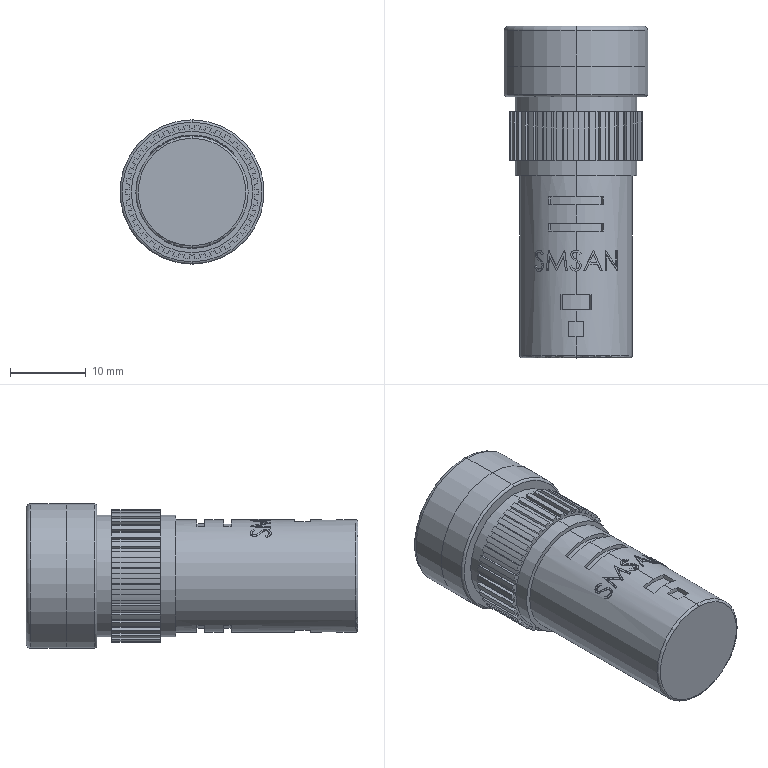Part | SolidWorks | features BaseBody 2 | 2 solids | 297 faces | box 19 x 43.7 x 19 mm | volume 9001 mm3 | plane 134 | cylinder 107 | spline 50 | torus 6 | commonest cylinder face diameters 16.6 x39 17.5 x38 13.8 x12 14.8 x5 15 x5 16 x4